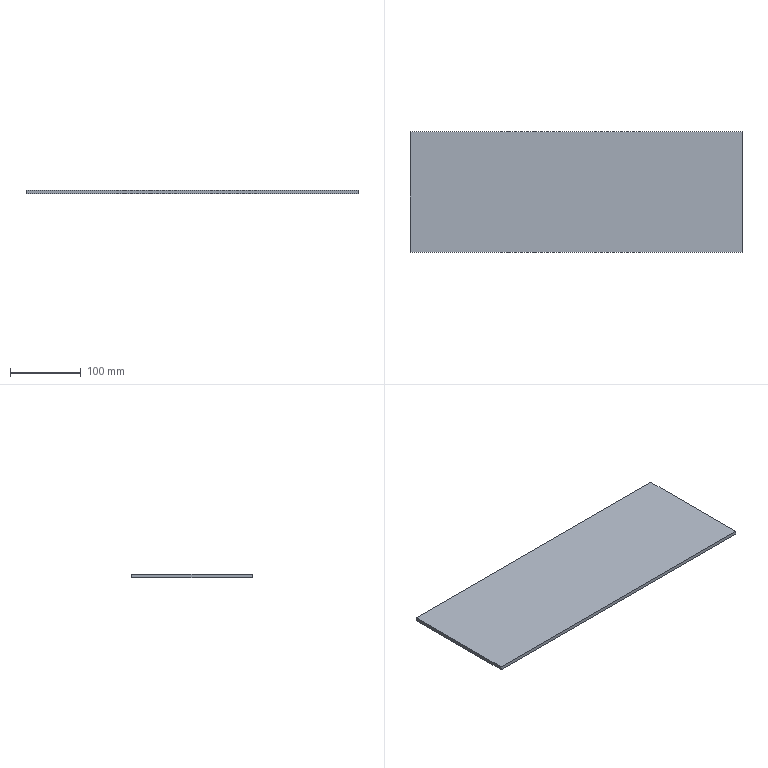Part | SolidWorks | features Extrusion 1 | 1 solid | 6 faces | box 470 x 170 x 5 mm | volume 399500 mm3 | plane 6
STEP:
#1=CARTESIAN_POINT('',(0.,0.,0.));
#2=VERTEX_POINT('',#1);
#3=CARTESIAN_POINT('',(470.,0.,0.));
#4=VERTEX_POINT('',#3);
#5=CARTESIAN_POINT('',(470.,0.,0.));
#6=DIRECTION('',(1.,0.,0.));
#7=VECTOR('',#6,1000.);
#8=LINE('',#5,#7);
#9=EDGE_CURVE('',#2,#4,#8,.T.);
#10=ORIENTED_EDGE('',*,*,#9,.T.);
#11=CARTESIAN_POINT('',(470.,0.,5.));
#12=VERTEX_POINT('',#11);
#13=CARTESIAN_POINT('',(470.,0.,5.));
#14=DIRECTION('',(0.,0.,-1.));
#15=VECTOR('',#14,1000.);
#16=LINE('',#13,#15);
#17=EDGE_CURVE('',#12,#4,#16,.T.);
#18=ORIENTED_EDGE('',*,*,#17,.F.);
#19=CARTESIAN_POINT('',(0.,0.,5.));
#20=VERTEX_POINT('',#19);
#21=CARTESIAN_POINT('',(470.,0.,5.));
#22=DIRECTION('',(1.,0.,0.));
#23=VECTOR('',#22,1000.);
#24=LINE('',#21,#23);
#25=EDGE_CURVE('',#20,#12,#24,.T.);
#26=ORIENTED_EDGE('',*,*,#25,.F.);
#27=CARTESIAN_POINT('',(0.,0.,5.));
#28=DIRECTION('',(0.,0.,-1.));
#29=VECTOR('',#28,1000.);
#30=LINE('',#27,#29);
#31=EDGE_CURVE('',#20,#2,#30,.T.);
#32=ORIENTED_EDGE('',*,*,#31,.T.);
#33=EDGE_LOOP('',(#10,#18,#26,#32));
#34=FACE_OUTER_BOUND('',#33,.T.);
#35=CARTESIAN_POINT('',(470.,0.,5.));
#36=DIRECTION('',(0.,1.,0.));
#37=DIRECTION('',(0.,0.,1.));
#38=AXIS2_PLACEMENT_3D('',#35,#36,#37);
#39=PLANE('',#38);
#40=ADVANCED_FACE('',(#34),#39,.F.);
#41=CARTESIAN_POINT('',(470.,170.,0.));
#42=VERTEX_POINT('',#41);
#43=CARTESIAN_POINT('',(470.,170.,0.));
#44=DIRECTION('',(0.,1.,0.));
#45=VECTOR('',#44,1000.);
#46=LINE('',#43,#45);
#47=EDGE_CURVE('',#4,#42,#46,.T.);
#48=ORIENTED_EDGE('',*,*,#47,.T.);
#49=CARTESIAN_POINT('',(470.,170.,5.));
#50=VERTEX_POINT('',#49);
#51=CARTESIAN_POINT('',(470.,170.,5.));
#52=DIRECTION('',(0.,0.,-1.));
#53=VECTOR('',#52,1000.);
#54=LINE('',#51,#53);
#55=EDGE_CURVE('',#50,#42,#54,.T.);
#56=ORIENTED_EDGE('',*,*,#55,.F.);
#57=CARTESIAN_POINT('',(470.,170.,5.));
#58=DIRECTION('',(0.,1.,0.));
#59=VECTOR('',#58,1000.);
#60=LINE('',#57,#59);
#61=EDGE_CURVE('',#12,#50,#60,.T.);
#62=ORIENTED_EDGE('',*,*,#61,.F.);
#63=ORIENTED_EDGE('',*,*,#17,.T.);
#64=EDGE_LOOP('',(#48,#56,#62,#63));
#65=FACE_OUTER_BOUND('',#64,.T.);
#66=CARTESIAN_POINT('',(470.,170.,5.));
#67=DIRECTION('',(-1.,0.,0.));
#68=DIRECTION('',(0.,0.,1.));
#69=AXIS2_PLACEMENT_3D('',#66,#67,#68);
#70=PLANE('',#69);
#71=ADVANCED_FACE('',(#65),#70,.F.);
#72=CARTESIAN_POINT('',(0.,170.,0.));
#73=VERTEX_POINT('',#72);
#74=CARTESIAN_POINT('',(0.,170.,0.));
#75=DIRECTION('',(-1.,0.,0.));
#76=VECTOR('',#75,1000.);
#77=LINE('',#74,#76);
#78=EDGE_CURVE('',#42,#73,#77,.T.);
#79=ORIENTED_EDGE('',*,*,#78,.T.);
#80=CARTESIAN_POINT('',(0.,170.,5.));
#81=VERTEX_POINT('',#80);
#82=CARTESIAN_POINT('',(0.,170.,5.));
#83=DIRECTION('',(0.,0.,-1.));
#84=VECTOR('',#83,1000.);
#85=LINE('',#82,#84);
#86=EDGE_CURVE('',#81,#73,#85,.T.);
#87=ORIENTED_EDGE('',*,*,#86,.F.);
#88=CARTESIAN_POINT('',(0.,170.,5.));
#89=DIRECTION('',(-1.,0.,0.));
#90=VECTOR('',#89,1000.);
#91=LINE('',#88,#90);
#92=EDGE_CURVE('',#50,#81,#91,.T.);
#93=ORIENTED_EDGE('',*,*,#92,.F.);
#94=ORIENTED_EDGE('',*,*,#55,.T.);
#95=EDGE_LOOP('',(#79,#87,#93,#94));
#96=FACE_OUTER_BOUND('',#95,.T.);
#97=CARTESIAN_POINT('',(0.,170.,5.));
#98=DIRECTION('',(0.,-1.,0.));
#99=DIRECTION('',(0.,0.,-1.));
#100=AXIS2_PLACEMENT_3D('',#97,#98,#99);
#101=PLANE('',#100);
#102=ADVANCED_FACE('',(#96),#101,.F.);
#103=CARTESIAN_POINT('',(0.,0.,0.));
#104=DIRECTION('',(0.,-1.,0.));
#105=VECTOR('',#104,1000.);
#106=LINE('',#103,#105);
#107=EDGE_CURVE('',#73,#2,#106,.T.);
#108=ORIENTED_EDGE('',*,*,#107,.T.);
#109=ORIENTED_EDGE('',*,*,#31,.F.);
#110=CARTESIAN_POINT('',(0.,0.,5.));
#111=DIRECTION('',(0.,-1.,0.));
#112=VECTOR('',#111,1000.);
#113=LINE('',#110,#112);
#114=EDGE_CURVE('',#81,#20,#113,.T.);
#115=ORIENTED_EDGE('',*,*,#114,.F.);
#116=ORIENTED_EDGE('',*,*,#86,.T.);
#117=EDGE_LOOP('',(#108,#109,#115,#116));
#118=FACE_OUTER_BOUND('',#117,.T.);
#119=CARTESIAN_POINT('',(0.,0.,5.));
#120=DIRECTION('',(1.,0.,0.));
#121=DIRECTION('',(0.,0.,-1.));
#122=AXIS2_PLACEMENT_3D('',#119,#120,#121);
#123=PLANE('',#122);
#124=ADVANCED_FACE('',(#118),#123,.F.);
#125=ORIENTED_EDGE('',*,*,#25,.T.);
#126=ORIENTED_EDGE('',*,*,#61,.T.);
#127=ORIENTED_EDGE('',*,*,#92,.T.);
#128=ORIENTED_EDGE('',*,*,#114,.T.);
#129=EDGE_LOOP('',(#125,#126,#127,#128));
#130=FACE_OUTER_BOUND('',#129,.T.);
#131=CARTESIAN_POINT('',(0.,0.,5.));
#132=DIRECTION('',(0.,0.,-1.));
#133=DIRECTION('',(-1.,0.,0.));
#134=AXIS2_PLACEMENT_3D('',#131,#132,#133);
#135=PLANE('',#134);
#136=ADVANCED_FACE('',(#130),#135,.F.);
#137=ORIENTED_EDGE('',*,*,#9,.F.);
#138=ORIENTED_EDGE('',*,*,#107,.F.);
#139=ORIENTED_EDGE('',*,*,#78,.F.);
#140=ORIENTED_EDGE('',*,*,#47,.F.);
#141=EDGE_LOOP('',(#137,#138,#139,#140));
#142=FACE_OUTER_BOUND('',#141,.T.);
#143=CARTESIAN_POINT('',(0.,0.,0.));
#144=DIRECTION('',(0.,0.,-1.));
#145=DIRECTION('',(-1.,0.,0.));
#146=AXIS2_PLACEMENT_3D('',#143,#144,#145);
#147=PLANE('',#146);
#148=ADVANCED_FACE('',(#142),#147,.T.);
#149=CLOSED_SHELL('',(#40,#71,#102,#124,#136,#148));
#150=MANIFOLD_SOLID_BREP('',#149);
#151=CARTESIAN_POINT('',(0.,0.,0.));
#152=DIRECTION('',(0.,0.,1.));
#153=DIRECTION('',(1.,0.,0.));
#154=AXIS2_PLACEMENT_3D('',#151,#152,#153);
#155=(LENGTH_UNIT()NAMED_UNIT(*)SI_UNIT(.MILLI.,.METRE.));
#156=UNCERTAINTY_MEASURE_WITH_UNIT(LENGTH_MEASURE(0.00001),#155,'','');
#157=(NAMED_UNIT(*)PLANE_ANGLE_UNIT()SI_UNIT($,.RADIAN.));
#158=(NAMED_UNIT(*)SI_UNIT($,.STERADIAN.)SOLID_ANGLE_UNIT());
#159=(GEOMETRIC_REPRESENTATION_CONTEXT(3)GLOBAL_UNCERTAINTY_ASSIGNED_CONTEXT((#156))GLOBAL_UNIT_ASSIGNED_CONTEXT((#155,#157,#158))REPRESENTATION_CONTEXT('',''));
#160=ADVANCED_BREP_SHAPE_REPRESENTATION('',(#150,#154),#159);